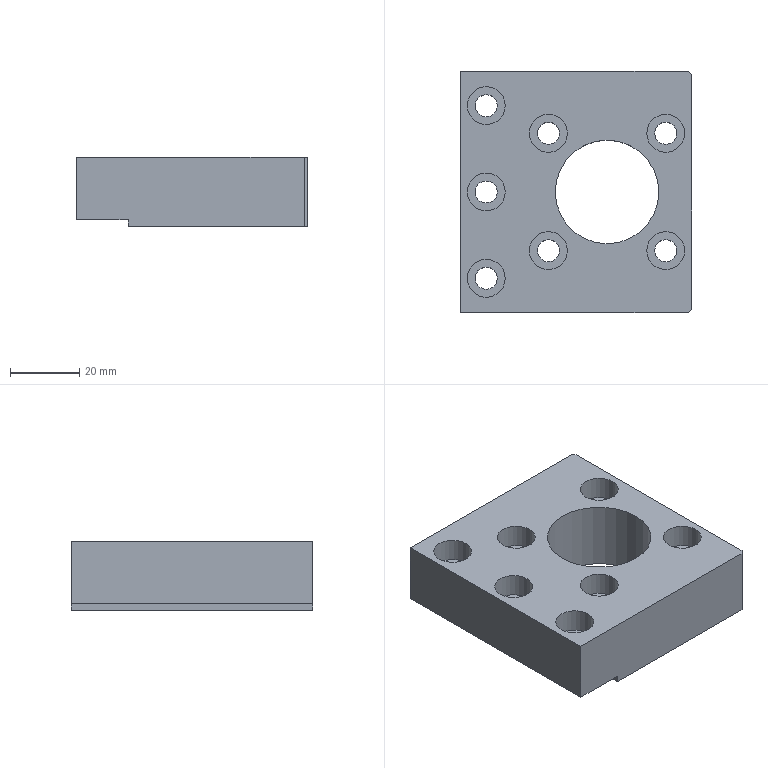Part | NX | 1 solid | 32 faces | box 67 x 70 x 20 mm | volume 70240 mm3 | plane 17 | cylinder 15 | commonest cylinder face diameters 6.4 x7 11 x7 30 x1
STEP:
#1=CARTESIAN_POINT('',(33.5,-34.,-10.));
#2=VERTEX_POINT('',#1);
#3=CARTESIAN_POINT('',(33.5,34.,-10.));
#4=VERTEX_POINT('',#3);
#5=CARTESIAN_POINT('',(33.5,35.,-10.));
#6=DIRECTION('',(0.,1.,0.));
#7=VECTOR('',#6,1000.);
#8=LINE('',#5,#7);
#9=EDGE_CURVE('',#2,#4,#8,.T.);
#10=ORIENTED_EDGE('',*,*,#9,.T.);
#11=CARTESIAN_POINT('',(33.5,34.,10.));
#12=VERTEX_POINT('',#11);
#13=CARTESIAN_POINT('',(33.5,34.,10.));
#14=DIRECTION('',(0.,0.,1.));
#15=VECTOR('',#14,1000.);
#16=LINE('',#13,#15);
#17=EDGE_CURVE('',#4,#12,#16,.T.);
#18=ORIENTED_EDGE('',*,*,#17,.T.);
#19=CARTESIAN_POINT('',(33.5,-34.,10.));
#20=VERTEX_POINT('',#19);
#21=CARTESIAN_POINT('',(33.5,35.,10.));
#22=DIRECTION('',(0.,1.,0.));
#23=VECTOR('',#22,1000.);
#24=LINE('',#21,#23);
#25=EDGE_CURVE('',#20,#12,#24,.T.);
#26=ORIENTED_EDGE('',*,*,#25,.F.);
#27=CARTESIAN_POINT('',(33.5,-34.,10.));
#28=DIRECTION('',(0.,0.,-1.));
#29=VECTOR('',#28,1000.);
#30=LINE('',#27,#29);
#31=EDGE_CURVE('',#20,#2,#30,.T.);
#32=ORIENTED_EDGE('',*,*,#31,.T.);
#33=EDGE_LOOP('',(#10,#18,#26,#32));
#34=FACE_BOUND('',#33,.T.);
#35=CARTESIAN_POINT('',(33.5,35.,10.));
#36=DIRECTION('',(-1.,0.,0.));
#37=DIRECTION('',(0.,-1.,0.));
#38=AXIS2_PLACEMENT_3D('',#35,#36,#37);
#39=PLANE('',#38);
#40=ADVANCED_FACE('',(#34),#39,.F.);
#41=CARTESIAN_POINT('',(32.5,35.,-10.));
#42=VERTEX_POINT('',#41);
#43=CARTESIAN_POINT('',(-18.5,35.,-10.));
#44=VERTEX_POINT('',#43);
#45=CARTESIAN_POINT('',(-33.5,35.,-10.));
#46=DIRECTION('',(-1.,0.,0.));
#47=VECTOR('',#46,1000.);
#48=LINE('',#45,#47);
#49=EDGE_CURVE('',#42,#44,#48,.T.);
#50=ORIENTED_EDGE('',*,*,#49,.T.);
#51=CARTESIAN_POINT('',(-18.5,35.,-8.));
#52=VERTEX_POINT('',#51);
#53=CARTESIAN_POINT('',(-18.5,35.,-10.));
#54=DIRECTION('',(0.,0.,-1.));
#55=VECTOR('',#54,1000.);
#56=LINE('',#53,#55);
#57=EDGE_CURVE('',#52,#44,#56,.T.);
#58=ORIENTED_EDGE('',*,*,#57,.F.);
#59=CARTESIAN_POINT('',(-33.5,35.,-8.));
#60=VERTEX_POINT('',#59);
#61=CARTESIAN_POINT('',(-33.5,35.,-8.));
#62=DIRECTION('',(1.,0.,0.));
#63=VECTOR('',#62,1000.);
#64=LINE('',#61,#63);
#65=EDGE_CURVE('',#60,#52,#64,.T.);
#66=ORIENTED_EDGE('',*,*,#65,.F.);
#67=CARTESIAN_POINT('',(-33.5,35.,10.));
#68=VERTEX_POINT('',#67);
#69=CARTESIAN_POINT('',(-33.5,35.,10.));
#70=DIRECTION('',(0.,0.,-1.));
#71=VECTOR('',#70,1000.);
#72=LINE('',#69,#71);
#73=EDGE_CURVE('',#68,#60,#72,.T.);
#74=ORIENTED_EDGE('',*,*,#73,.F.);
#75=CARTESIAN_POINT('',(32.5,35.,10.));
#76=VERTEX_POINT('',#75);
#77=CARTESIAN_POINT('',(-33.5,35.,10.));
#78=DIRECTION('',(-1.,0.,0.));
#79=VECTOR('',#78,1000.);
#80=LINE('',#77,#79);
#81=EDGE_CURVE('',#76,#68,#80,.T.);
#82=ORIENTED_EDGE('',*,*,#81,.F.);
#83=CARTESIAN_POINT('',(32.5,35.,10.));
#84=DIRECTION('',(0.,0.,-1.));
#85=VECTOR('',#84,1000.);
#86=LINE('',#83,#85);
#87=EDGE_CURVE('',#76,#42,#86,.T.);
#88=ORIENTED_EDGE('',*,*,#87,.T.);
#89=EDGE_LOOP('',(#50,#58,#66,#74,#82,#88));
#90=FACE_BOUND('',#89,.T.);
#91=CARTESIAN_POINT('',(-33.5,35.,10.));
#92=DIRECTION('',(0.,-1.,0.));
#93=DIRECTION('',(0.,0.,-1.));
#94=AXIS2_PLACEMENT_3D('',#91,#92,#93);
#95=PLANE('',#94);
#96=ADVANCED_FACE('',(#90),#95,.F.);
#97=ORIENTED_EDGE('',*,*,#73,.T.);
#98=CARTESIAN_POINT('',(-33.5,-35.,-8.));
#99=VERTEX_POINT('',#98);
#100=CARTESIAN_POINT('',(-33.5,-35.,-8.));
#101=DIRECTION('',(0.,1.,0.));
#102=VECTOR('',#101,1000.);
#103=LINE('',#100,#102);
#104=EDGE_CURVE('',#99,#60,#103,.T.);
#105=ORIENTED_EDGE('',*,*,#104,.F.);
#106=CARTESIAN_POINT('',(-33.5,-35.,10.));
#107=VERTEX_POINT('',#106);
#108=CARTESIAN_POINT('',(-33.5,-35.,10.));
#109=DIRECTION('',(0.,0.,-1.));
#110=VECTOR('',#109,1000.);
#111=LINE('',#108,#110);
#112=EDGE_CURVE('',#107,#99,#111,.T.);
#113=ORIENTED_EDGE('',*,*,#112,.F.);
#114=CARTESIAN_POINT('',(-33.5,35.,10.));
#115=DIRECTION('',(0.,-1.,0.));
#116=VECTOR('',#115,1000.);
#117=LINE('',#114,#116);
#118=EDGE_CURVE('',#68,#107,#117,.T.);
#119=ORIENTED_EDGE('',*,*,#118,.F.);
#120=EDGE_LOOP('',(#97,#105,#113,#119));
#121=FACE_BOUND('',#120,.T.);
#122=CARTESIAN_POINT('',(-33.5,35.,10.));
#123=DIRECTION('',(1.,0.,0.));
#124=DIRECTION('',(0.,1.,0.));
#125=AXIS2_PLACEMENT_3D('',#122,#123,#124);
#126=PLANE('',#125);
#127=ADVANCED_FACE('',(#121),#126,.F.);
#128=CARTESIAN_POINT('',(-18.5,-35.,-8.));
#129=VERTEX_POINT('',#128);
#130=CARTESIAN_POINT('',(-33.5,-35.,-8.));
#131=DIRECTION('',(1.,0.,0.));
#132=VECTOR('',#131,1000.);
#133=LINE('',#130,#132);
#134=EDGE_CURVE('',#99,#129,#133,.T.);
#135=ORIENTED_EDGE('',*,*,#134,.T.);
#136=CARTESIAN_POINT('',(-18.5,-35.,-10.));
#137=VERTEX_POINT('',#136);
#138=CARTESIAN_POINT('',(-18.5,-35.,-10.));
#139=DIRECTION('',(0.,0.,-1.));
#140=VECTOR('',#139,1000.);
#141=LINE('',#138,#140);
#142=EDGE_CURVE('',#129,#137,#141,.T.);
#143=ORIENTED_EDGE('',*,*,#142,.T.);
#144=CARTESIAN_POINT('',(32.5,-35.,-10.));
#145=VERTEX_POINT('',#144);
#146=CARTESIAN_POINT('',(-33.5,-35.,-10.));
#147=DIRECTION('',(1.,0.,0.));
#148=VECTOR('',#147,1000.);
#149=LINE('',#146,#148);
#150=EDGE_CURVE('',#137,#145,#149,.T.);
#151=ORIENTED_EDGE('',*,*,#150,.T.);
#152=CARTESIAN_POINT('',(32.5,-35.,10.));
#153=VERTEX_POINT('',#152);
#154=CARTESIAN_POINT('',(32.5,-35.,10.));
#155=DIRECTION('',(0.,0.,1.));
#156=VECTOR('',#155,1000.);
#157=LINE('',#154,#156);
#158=EDGE_CURVE('',#145,#153,#157,.T.);
#159=ORIENTED_EDGE('',*,*,#158,.T.);
#160=CARTESIAN_POINT('',(-33.5,-35.,10.));
#161=DIRECTION('',(1.,0.,0.));
#162=VECTOR('',#161,1000.);
#163=LINE('',#160,#162);
#164=EDGE_CURVE('',#107,#153,#163,.T.);
#165=ORIENTED_EDGE('',*,*,#164,.F.);
#166=ORIENTED_EDGE('',*,*,#112,.T.);
#167=EDGE_LOOP('',(#135,#143,#151,#159,#165,#166));
#168=FACE_BOUND('',#167,.T.);
#169=CARTESIAN_POINT('',(-33.5,-35.,10.));
#170=DIRECTION('',(0.,1.,0.));
#171=DIRECTION('',(0.,0.,1.));
#172=AXIS2_PLACEMENT_3D('',#169,#170,#171);
#173=PLANE('',#172);
#174=ADVANCED_FACE('',(#168),#173,.F.);
#175=CARTESIAN_POINT('',(-20.5,25.,10.));
#176=VERTEX_POINT('',#175);
#177=CARTESIAN_POINT('',(-26.,25.,10.));
#178=DIRECTION('',(0.,0.,1.));
#179=DIRECTION('',(1.,0.,0.));
#180=AXIS2_PLACEMENT_3D('',#177,#178,#179);
#181=CIRCLE('',#180,5.5);
#182=EDGE_CURVE('',#176,#176,#181,.T.);
#183=ORIENTED_EDGE('',*,*,#182,.F.);
#184=EDGE_LOOP('',(#183));
#185=FACE_BOUND('',#184,.T.);
#186=CARTESIAN_POINT('',(-20.5,0.,10.));
#187=VERTEX_POINT('',#186);
#188=CARTESIAN_POINT('',(-26.,0.,10.));
#189=DIRECTION('',(0.,0.,1.));
#190=DIRECTION('',(1.,0.,0.));
#191=AXIS2_PLACEMENT_3D('',#188,#189,#190);
#192=CIRCLE('',#191,5.5);
#193=EDGE_CURVE('',#187,#187,#192,.T.);
#194=ORIENTED_EDGE('',*,*,#193,.F.);
#195=EDGE_LOOP('',(#194));
#196=FACE_BOUND('',#195,.T.);
#197=CARTESIAN_POINT('',(-20.5,-25.,10.));
#198=VERTEX_POINT('',#197);
#199=CARTESIAN_POINT('',(-26.,-25.,10.));
#200=DIRECTION('',(0.,0.,1.));
#201=DIRECTION('',(1.,0.,0.));
#202=AXIS2_PLACEMENT_3D('',#199,#200,#201);
#203=CIRCLE('',#202,5.5);
#204=EDGE_CURVE('',#198,#198,#203,.T.);
#205=ORIENTED_EDGE('',*,*,#204,.F.);
#206=EDGE_LOOP('',(#205));
#207=FACE_BOUND('',#206,.T.);
#208=CARTESIAN_POINT('',(-2.5,-17.,10.));
#209=VERTEX_POINT('',#208);
#210=CARTESIAN_POINT('',(-8.,-17.,10.));
#211=DIRECTION('',(0.,0.,1.));
#212=DIRECTION('',(1.,0.,0.));
#213=AXIS2_PLACEMENT_3D('',#210,#211,#212);
#214=CIRCLE('',#213,5.5);
#215=EDGE_CURVE('',#209,#209,#214,.T.);
#216=ORIENTED_EDGE('',*,*,#215,.F.);
#217=EDGE_LOOP('',(#216));
#218=FACE_BOUND('',#217,.T.);
#219=CARTESIAN_POINT('',(-2.5,17.,10.));
#220=VERTEX_POINT('',#219);
#221=CARTESIAN_POINT('',(-8.,17.,10.));
#222=DIRECTION('',(0.,0.,1.));
#223=DIRECTION('',(1.,0.,0.));
#224=AXIS2_PLACEMENT_3D('',#221,#222,#223);
#225=CIRCLE('',#224,5.5);
#226=EDGE_CURVE('',#220,#220,#225,.T.);
#227=ORIENTED_EDGE('',*,*,#226,.F.);
#228=EDGE_LOOP('',(#227));
#229=FACE_BOUND('',#228,.T.);
#230=CARTESIAN_POINT('',(31.5,17.,10.));
#231=VERTEX_POINT('',#230);
#232=CARTESIAN_POINT('',(26.,17.,10.));
#233=DIRECTION('',(0.,0.,1.));
#234=DIRECTION('',(1.,0.,0.));
#235=AXIS2_PLACEMENT_3D('',#232,#233,#234);
#236=CIRCLE('',#235,5.5);
#237=EDGE_CURVE('',#231,#231,#236,.T.);
#238=ORIENTED_EDGE('',*,*,#237,.F.);
#239=EDGE_LOOP('',(#238));
#240=FACE_BOUND('',#239,.T.);
#241=CARTESIAN_POINT('',(31.5,-17.,10.));
#242=VERTEX_POINT('',#241);
#243=CARTESIAN_POINT('',(26.,-17.,10.));
#244=DIRECTION('',(0.,0.,1.));
#245=DIRECTION('',(1.,0.,0.));
#246=AXIS2_PLACEMENT_3D('',#243,#244,#245);
#247=CIRCLE('',#246,5.5);
#248=EDGE_CURVE('',#242,#242,#247,.T.);
#249=ORIENTED_EDGE('',*,*,#248,.F.);
#250=EDGE_LOOP('',(#249));
#251=FACE_BOUND('',#250,.T.);
#252=CARTESIAN_POINT('',(-6.,0.,10.));
#253=VERTEX_POINT('',#252);
#254=CARTESIAN_POINT('',(9.,0.,10.));
#255=DIRECTION('',(0.,0.,-1.));
#256=DIRECTION('',(-1.,0.,0.));
#257=AXIS2_PLACEMENT_3D('',#254,#255,#256);
#258=CIRCLE('',#257,15.);
#259=EDGE_CURVE('',#253,#253,#258,.T.);
#260=ORIENTED_EDGE('',*,*,#259,.T.);
#261=EDGE_LOOP('',(#260));
#262=FACE_BOUND('',#261,.T.);
#263=ORIENTED_EDGE('',*,*,#25,.T.);
#264=CARTESIAN_POINT('',(33.75,33.75,10.));
#265=DIRECTION('',(0.7071,-0.7071,0.));
#266=VECTOR('',#265,1000.);
#267=LINE('',#264,#266);
#268=EDGE_CURVE('',#12,#76,#267,.F.);
#269=ORIENTED_EDGE('',*,*,#268,.T.);
#270=ORIENTED_EDGE('',*,*,#81,.T.);
#271=ORIENTED_EDGE('',*,*,#118,.T.);
#272=ORIENTED_EDGE('',*,*,#164,.T.);
#273=CARTESIAN_POINT('',(33.75,-33.75,10.));
#274=DIRECTION('',(-0.7071,-0.7071,0.));
#275=VECTOR('',#274,1000.);
#276=LINE('',#273,#275);
#277=EDGE_CURVE('',#153,#20,#276,.F.);
#278=ORIENTED_EDGE('',*,*,#277,.T.);
#279=EDGE_LOOP('',(#263,#269,#270,#271,#272,#278));
#280=FACE_BOUND('',#279,.T.);
#281=CARTESIAN_POINT('',(0.,0.,10.));
#282=DIRECTION('',(0.,0.,1.));
#283=DIRECTION('',(1.,0.,0.));
#284=AXIS2_PLACEMENT_3D('',#281,#282,#283);
#285=PLANE('',#284);
#286=ADVANCED_FACE('',(#185,#196,#207,#218,#229,#240,#251,#262,#280),#285,.T.);
#287=CARTESIAN_POINT('',(-4.8,-17.,-10.));
#288=VERTEX_POINT('',#287);
#289=CARTESIAN_POINT('',(-8.,-17.,-10.));
#290=DIRECTION('',(0.,0.,1.));
#291=DIRECTION('',(1.,0.,0.));
#292=AXIS2_PLACEMENT_3D('',#289,#290,#291);
#293=CIRCLE('',#292,3.2);
#294=EDGE_CURVE('',#288,#288,#293,.T.);
#295=ORIENTED_EDGE('',*,*,#294,.T.);
#296=EDGE_LOOP('',(#295));
#297=FACE_BOUND('',#296,.T.);
#298=CARTESIAN_POINT('',(-4.8,17.,-10.));
#299=VERTEX_POINT('',#298);
#300=CARTESIAN_POINT('',(-8.,17.,-10.));
#301=DIRECTION('',(0.,0.,1.));
#302=DIRECTION('',(1.,0.,0.));
#303=AXIS2_PLACEMENT_3D('',#300,#301,#302);
#304=CIRCLE('',#303,3.2);
#305=EDGE_CURVE('',#299,#299,#304,.T.);
#306=ORIENTED_EDGE('',*,*,#305,.T.);
#307=EDGE_LOOP('',(#306));
#308=FACE_BOUND('',#307,.T.);
#309=CARTESIAN_POINT('',(29.2,17.,-10.));
#310=VERTEX_POINT('',#309);
#311=CARTESIAN_POINT('',(26.,17.,-10.));
#312=DIRECTION('',(0.,0.,1.));
#313=DIRECTION('',(1.,0.,0.));
#314=AXIS2_PLACEMENT_3D('',#311,#312,#313);
#315=CIRCLE('',#314,3.2);
#316=EDGE_CURVE('',#310,#310,#315,.T.);
#317=ORIENTED_EDGE('',*,*,#316,.T.);
#318=EDGE_LOOP('',(#317));
#319=FACE_BOUND('',#318,.T.);
#320=CARTESIAN_POINT('',(29.2,-17.,-10.));
#321=VERTEX_POINT('',#320);
#322=CARTESIAN_POINT('',(26.,-17.,-10.));
#323=DIRECTION('',(0.,0.,1.));
#324=DIRECTION('',(1.,0.,0.));
#325=AXIS2_PLACEMENT_3D('',#322,#323,#324);
#326=CIRCLE('',#325,3.2);
#327=EDGE_CURVE('',#321,#321,#326,.T.);
#328=ORIENTED_EDGE('',*,*,#327,.T.);
#329=EDGE_LOOP('',(#328));
#330=FACE_BOUND('',#329,.T.);
#331=CARTESIAN_POINT('',(-6.,0.,-10.));
#332=VERTEX_POINT('',#331);
#333=CARTESIAN_POINT('',(9.,0.,-10.));
#334=DIRECTION('',(0.,0.,-1.));
#335=DIRECTION('',(-1.,0.,0.));
#336=AXIS2_PLACEMENT_3D('',#333,#334,#335);
#337=CIRCLE('',#336,15.);
#338=EDGE_CURVE('',#332,#332,#337,.T.);
#339=ORIENTED_EDGE('',*,*,#338,.F.);
#340=EDGE_LOOP('',(#339));
#341=FACE_BOUND('',#340,.T.);
#342=ORIENTED_EDGE('',*,*,#150,.F.);
#343=CARTESIAN_POINT('',(-18.5,-35.,-10.));
#344=DIRECTION('',(0.,1.,0.));
#345=VECTOR('',#344,1000.);
#346=LINE('',#343,#345);
#347=EDGE_CURVE('',#137,#44,#346,.T.);
#348=ORIENTED_EDGE('',*,*,#347,.T.);
#349=ORIENTED_EDGE('',*,*,#49,.F.);
#350=CARTESIAN_POINT('',(32.5,35.,-10.));
#351=DIRECTION('',(-0.7071,0.7071,0.));
#352=VECTOR('',#351,1000.);
#353=LINE('',#350,#352);
#354=EDGE_CURVE('',#42,#4,#353,.F.);
#355=ORIENTED_EDGE('',*,*,#354,.T.);
#356=ORIENTED_EDGE('',*,*,#9,.F.);
#357=CARTESIAN_POINT('',(33.5,-34.,-10.));
#358=DIRECTION('',(0.7071,0.7071,0.));
#359=VECTOR('',#358,1000.);
#360=LINE('',#357,#359);
#361=EDGE_CURVE('',#2,#145,#360,.F.);
#362=ORIENTED_EDGE('',*,*,#361,.T.);
#363=EDGE_LOOP('',(#342,#348,#349,#355,#356,#362));
#364=FACE_BOUND('',#363,.T.);
#365=CARTESIAN_POINT('',(0.,0.,-10.));
#366=DIRECTION('',(0.,0.,1.));
#367=DIRECTION('',(1.,0.,0.));
#368=AXIS2_PLACEMENT_3D('',#365,#366,#367);
#369=PLANE('',#368);
#370=ADVANCED_FACE('',(#297,#308,#319,#330,#341,#364),#369,.F.);
#371=ORIENTED_EDGE('',*,*,#259,.F.);
#372=EDGE_LOOP('',(#371));
#373=FACE_BOUND('',#372,.T.);
#374=ORIENTED_EDGE('',*,*,#338,.T.);
#375=EDGE_LOOP('',(#374));
#376=FACE_BOUND('',#375,.T.);
#377=CARTESIAN_POINT('',(9.,0.,10.));
#378=DIRECTION('',(0.,0.,-1.));
#379=DIRECTION('',(-1.,0.,0.));
#380=AXIS2_PLACEMENT_3D('',#377,#378,#379);
#381=CYLINDRICAL_SURFACE('',#380,15.);
#382=ADVANCED_FACE('',(#373,#376),#381,.F.);
#383=ORIENTED_EDGE('',*,*,#268,.F.);
#384=ORIENTED_EDGE('',*,*,#17,.F.);
#385=ORIENTED_EDGE('',*,*,#354,.F.);
#386=ORIENTED_EDGE('',*,*,#87,.F.);
#387=EDGE_LOOP('',(#383,#384,#385,#386));
#388=FACE_BOUND('',#387,.T.);
#389=CARTESIAN_POINT('',(32.5,35.,10.));
#390=DIRECTION('',(-0.7071,-0.7071,0.));
#391=DIRECTION('',(0.,0.,-1.));
#392=AXIS2_PLACEMENT_3D('',#389,#390,#391);
#393=PLANE('',#392);
#394=ADVANCED_FACE('',(#388),#393,.F.);
#395=ORIENTED_EDGE('',*,*,#277,.F.);
#396=ORIENTED_EDGE('',*,*,#158,.F.);
#397=ORIENTED_EDGE('',*,*,#361,.F.);
#398=ORIENTED_EDGE('',*,*,#31,.F.);
#399=EDGE_LOOP('',(#395,#396,#397,#398));
#400=FACE_BOUND('',#399,.T.);
#401=CARTESIAN_POINT('',(33.5,-34.,10.));
#402=DIRECTION('',(-0.7071,0.7071,0.));
#403=DIRECTION('',(0.,0.,-1.));
#404=AXIS2_PLACEMENT_3D('',#401,#402,#403);
#405=PLANE('',#404);
#406=ADVANCED_FACE('',(#400),#405,.F.);
#407=ORIENTED_EDGE('',*,*,#327,.F.);
#408=EDGE_LOOP('',(#407));
#409=FACE_BOUND('',#408,.T.);
#410=CARTESIAN_POINT('',(29.2,-17.,3.2));
#411=VERTEX_POINT('',#410);
#412=CARTESIAN_POINT('',(26.,-17.,3.2));
#413=DIRECTION('',(0.,0.,1.));
#414=DIRECTION('',(1.,0.,0.));
#415=AXIS2_PLACEMENT_3D('',#412,#413,#414);
#416=CIRCLE('',#415,3.2);
#417=EDGE_CURVE('',#411,#411,#416,.T.);
#418=ORIENTED_EDGE('',*,*,#417,.T.);
#419=EDGE_LOOP('',(#418));
#420=FACE_BOUND('',#419,.T.);
#421=CARTESIAN_POINT('',(26.,-17.,10.));
#422=DIRECTION('',(0.,0.,1.));
#423=DIRECTION('',(1.,0.,0.));
#424=AXIS2_PLACEMENT_3D('',#421,#422,#423);
#425=CYLINDRICAL_SURFACE('',#424,3.2);
#426=ADVANCED_FACE('',(#409,#420),#425,.F.);
#427=ORIENTED_EDGE('',*,*,#417,.F.);
#428=EDGE_LOOP('',(#427));
#429=FACE_BOUND('',#428,.T.);
#430=CARTESIAN_POINT('',(31.5,-17.,3.2));
#431=VERTEX_POINT('',#430);
#432=CARTESIAN_POINT('',(26.,-17.,3.2));
#433=DIRECTION('',(0.,0.,1.));
#434=DIRECTION('',(1.,0.,0.));
#435=AXIS2_PLACEMENT_3D('',#432,#433,#434);
#436=CIRCLE('',#435,5.5);
#437=EDGE_CURVE('',#431,#431,#436,.T.);
#438=ORIENTED_EDGE('',*,*,#437,.T.);
#439=EDGE_LOOP('',(#438));
#440=FACE_BOUND('',#439,.T.);
#441=CARTESIAN_POINT('',(29.2,-17.,3.2));
#442=DIRECTION('',(0.,0.,-1.));
#443=DIRECTION('',(-1.,0.,0.));
#444=AXIS2_PLACEMENT_3D('',#441,#442,#443);
#445=PLANE('',#444);
#446=ADVANCED_FACE('',(#429,#440),#445,.F.);
#447=ORIENTED_EDGE('',*,*,#437,.F.);
#448=EDGE_LOOP('',(#447));
#449=FACE_BOUND('',#448,.T.);
#450=ORIENTED_EDGE('',*,*,#248,.T.);
#451=EDGE_LOOP('',(#450));
#452=FACE_BOUND('',#451,.T.);
#453=CARTESIAN_POINT('',(26.,-17.,10.));
#454=DIRECTION('',(0.,0.,1.));
#455=DIRECTION('',(1.,0.,0.));
#456=AXIS2_PLACEMENT_3D('',#453,#454,#455);
#457=CYLINDRICAL_SURFACE('',#456,5.5);
#458=ADVANCED_FACE('',(#449,#452),#457,.F.);
#459=ORIENTED_EDGE('',*,*,#316,.F.);
#460=EDGE_LOOP('',(#459));
#461=FACE_BOUND('',#460,.T.);
#462=CARTESIAN_POINT('',(29.2,17.,3.2));
#463=VERTEX_POINT('',#462);
#464=CARTESIAN_POINT('',(26.,17.,3.2));
#465=DIRECTION('',(0.,0.,1.));
#466=DIRECTION('',(1.,0.,0.));
#467=AXIS2_PLACEMENT_3D('',#464,#465,#466);
#468=CIRCLE('',#467,3.2);
#469=EDGE_CURVE('',#463,#463,#468,.T.);
#470=ORIENTED_EDGE('',*,*,#469,.T.);
#471=EDGE_LOOP('',(#470));
#472=FACE_BOUND('',#471,.T.);
#473=CARTESIAN_POINT('',(26.,17.,10.));
#474=DIRECTION('',(0.,0.,1.));
#475=DIRECTION('',(1.,0.,0.));
#476=AXIS2_PLACEMENT_3D('',#473,#474,#475);
#477=CYLINDRICAL_SURFACE('',#476,3.2);
#478=ADVANCED_FACE('',(#461,#472),#477,.F.);
#479=ORIENTED_EDGE('',*,*,#469,.F.);
#480=EDGE_LOOP('',(#479));
#481=FACE_BOUND('',#480,.T.);
#482=CARTESIAN_POINT('',(31.5,17.,3.2));
#483=VERTEX_POINT('',#482);
#484=CARTESIAN_POINT('',(26.,17.,3.2));
#485=DIRECTION('',(0.,0.,1.));
#486=DIRECTION('',(1.,0.,0.));
#487=AXIS2_PLACEMENT_3D('',#484,#485,#486);
#488=CIRCLE('',#487,5.5);
#489=EDGE_CURVE('',#483,#483,#488,.T.);
#490=ORIENTED_EDGE('',*,*,#489,.T.);
#491=EDGE_LOOP('',(#490));
#492=FACE_BOUND('',#491,.T.);
#493=CARTESIAN_POINT('',(29.2,17.,3.2));
#494=DIRECTION('',(0.,0.,-1.));
#495=DIRECTION('',(-1.,0.,0.));
#496=AXIS2_PLACEMENT_3D('',#493,#494,#495);
#497=PLANE('',#496);
#498=ADVANCED_FACE('',(#481,#492),#497,.F.);
#499=ORIENTED_EDGE('',*,*,#489,.F.);
#500=EDGE_LOOP('',(#499));
#501=FACE_BOUND('',#500,.T.);
#502=ORIENTED_EDGE('',*,*,#237,.T.);
#503=EDGE_LOOP('',(#502));
#504=FACE_BOUND('',#503,.T.);
#505=CARTESIAN_POINT('',(26.,17.,10.));
#506=DIRECTION('',(0.,0.,1.));
#507=DIRECTION('',(1.,0.,0.));
#508=AXIS2_PLACEMENT_3D('',#505,#506,#507);
#509=CYLINDRICAL_SURFACE('',#508,5.5);
#510=ADVANCED_FACE('',(#501,#504),#509,.F.);
#511=ORIENTED_EDGE('',*,*,#305,.F.);
#512=EDGE_LOOP('',(#511));
#513=FACE_BOUND('',#512,.T.);
#514=CARTESIAN_POINT('',(-4.8,17.,3.2));
#515=VERTEX_POINT('',#514);
#516=CARTESIAN_POINT('',(-8.,17.,3.2));
#517=DIRECTION('',(0.,0.,1.));
#518=DIRECTION('',(1.,0.,0.));
#519=AXIS2_PLACEMENT_3D('',#516,#517,#518);
#520=CIRCLE('',#519,3.2);
#521=EDGE_CURVE('',#515,#515,#520,.T.);
#522=ORIENTED_EDGE('',*,*,#521,.T.);
#523=EDGE_LOOP('',(#522));
#524=FACE_BOUND('',#523,.T.);
#525=CARTESIAN_POINT('',(-8.,17.,10.));
#526=DIRECTION('',(0.,0.,1.));
#527=DIRECTION('',(1.,0.,0.));
#528=AXIS2_PLACEMENT_3D('',#525,#526,#527);
#529=CYLINDRICAL_SURFACE('',#528,3.2);
#530=ADVANCED_FACE('',(#513,#524),#529,.F.);
#531=ORIENTED_EDGE('',*,*,#521,.F.);
#532=EDGE_LOOP('',(#531));
#533=FACE_BOUND('',#532,.T.);
#534=CARTESIAN_POINT('',(-2.5,17.,3.2));
#535=VERTEX_POINT('',#534);
#536=CARTESIAN_POINT('',(-8.,17.,3.2));
#537=DIRECTION('',(0.,0.,1.));
#538=DIRECTION('',(1.,0.,0.));
#539=AXIS2_PLACEMENT_3D('',#536,#537,#538);
#540=CIRCLE('',#539,5.5);
#541=EDGE_CURVE('',#535,#535,#540,.T.);
#542=ORIENTED_EDGE('',*,*,#541,.T.);
#543=EDGE_LOOP('',(#542));
#544=FACE_BOUND('',#543,.T.);
#545=CARTESIAN_POINT('',(-4.8,17.,3.2));
#546=DIRECTION('',(0.,0.,-1.));
#547=DIRECTION('',(-1.,0.,0.));
#548=AXIS2_PLACEMENT_3D('',#545,#546,#547);
#549=PLANE('',#548);
#550=ADVANCED_FACE('',(#533,#544),#549,.F.);
#551=ORIENTED_EDGE('',*,*,#541,.F.);
#552=EDGE_LOOP('',(#551));
#553=FACE_BOUND('',#552,.T.);
#554=ORIENTED_EDGE('',*,*,#226,.T.);
#555=EDGE_LOOP('',(#554));
#556=FACE_BOUND('',#555,.T.);
#557=CARTESIAN_POINT('',(-8.,17.,10.));
#558=DIRECTION('',(0.,0.,1.));
#559=DIRECTION('',(1.,0.,0.));
#560=AXIS2_PLACEMENT_3D('',#557,#558,#559);
#561=CYLINDRICAL_SURFACE('',#560,5.5);
#562=ADVANCED_FACE('',(#553,#556),#561,.F.);
#563=ORIENTED_EDGE('',*,*,#294,.F.);
#564=EDGE_LOOP('',(#563));
#565=FACE_BOUND('',#564,.T.);
#566=CARTESIAN_POINT('',(-4.8,-17.,3.2));
#567=VERTEX_POINT('',#566);
#568=CARTESIAN_POINT('',(-8.,-17.,3.2));
#569=DIRECTION('',(0.,0.,1.));
#570=DIRECTION('',(1.,0.,0.));
#571=AXIS2_PLACEMENT_3D('',#568,#569,#570);
#572=CIRCLE('',#571,3.2);
#573=EDGE_CURVE('',#567,#567,#572,.T.);
#574=ORIENTED_EDGE('',*,*,#573,.T.);
#575=EDGE_LOOP('',(#574));
#576=FACE_BOUND('',#575,.T.);
#577=CARTESIAN_POINT('',(-8.,-17.,10.));
#578=DIRECTION('',(0.,0.,1.));
#579=DIRECTION('',(1.,0.,0.));
#580=AXIS2_PLACEMENT_3D('',#577,#578,#579);
#581=CYLINDRICAL_SURFACE('',#580,3.2);
#582=ADVANCED_FACE('',(#565,#576),#581,.F.);
#583=ORIENTED_EDGE('',*,*,#573,.F.);
#584=EDGE_LOOP('',(#583));
#585=FACE_BOUND('',#584,.T.);
#586=CARTESIAN_POINT('',(-2.5,-17.,3.2));
#587=VERTEX_POINT('',#586);
#588=CARTESIAN_POINT('',(-8.,-17.,3.2));
#589=DIRECTION('',(0.,0.,1.));
#590=DIRECTION('',(1.,0.,0.));
#591=AXIS2_PLACEMENT_3D('',#588,#589,#590);
#592=CIRCLE('',#591,5.5);
#593=EDGE_CURVE('',#587,#587,#592,.T.);
#594=ORIENTED_EDGE('',*,*,#593,.T.);
#595=EDGE_LOOP('',(#594));
#596=FACE_BOUND('',#595,.T.);
#597=CARTESIAN_POINT('',(-4.8,-17.,3.2));
#598=DIRECTION('',(0.,0.,-1.));
#599=DIRECTION('',(-1.,0.,0.));
#600=AXIS2_PLACEMENT_3D('',#597,#598,#599);
#601=PLANE('',#600);
#602=ADVANCED_FACE('',(#585,#596),#601,.F.);
#603=ORIENTED_EDGE('',*,*,#593,.F.);
#604=EDGE_LOOP('',(#603));
#605=FACE_BOUND('',#604,.T.);
#606=ORIENTED_EDGE('',*,*,#215,.T.);
#607=EDGE_LOOP('',(#606));
#608=FACE_BOUND('',#607,.T.);
#609=CARTESIAN_POINT('',(-8.,-17.,10.));
#610=DIRECTION('',(0.,0.,1.));
#611=DIRECTION('',(1.,0.,0.));
#612=AXIS2_PLACEMENT_3D('',#609,#610,#611);
#613=CYLINDRICAL_SURFACE('',#612,5.5);
#614=ADVANCED_FACE('',(#605,#608),#613,.F.);
#615=ORIENTED_EDGE('',*,*,#57,.T.);
#616=ORIENTED_EDGE('',*,*,#347,.F.);
#617=ORIENTED_EDGE('',*,*,#142,.F.);
#618=CARTESIAN_POINT('',(-18.5,-35.,-8.));
#619=DIRECTION('',(0.,1.,0.));
#620=VECTOR('',#619,1000.);
#621=LINE('',#618,#620);
#622=EDGE_CURVE('',#129,#52,#621,.T.);
#623=ORIENTED_EDGE('',*,*,#622,.T.);
#624=EDGE_LOOP('',(#615,#616,#617,#623));
#625=FACE_BOUND('',#624,.T.);
#626=CARTESIAN_POINT('',(-18.5,-35.,-10.));
#627=DIRECTION('',(1.,0.,0.));
#628=DIRECTION('',(0.,0.,-1.));
#629=AXIS2_PLACEMENT_3D('',#626,#627,#628);
#630=PLANE('',#629);
#631=ADVANCED_FACE('',(#625),#630,.F.);
#632=CARTESIAN_POINT('',(-22.8,25.,-8.));
#633=VERTEX_POINT('',#632);
#634=CARTESIAN_POINT('',(-26.,25.,-8.));
#635=DIRECTION('',(0.,0.,1.));
#636=DIRECTION('',(1.,0.,0.));
#637=AXIS2_PLACEMENT_3D('',#634,#635,#636);
#638=CIRCLE('',#637,3.2);
#639=EDGE_CURVE('',#633,#633,#638,.T.);
#640=ORIENTED_EDGE('',*,*,#639,.T.);
#641=EDGE_LOOP('',(#640));
#642=FACE_BOUND('',#641,.T.);
#643=CARTESIAN_POINT('',(-22.8,0.,-8.));
#644=VERTEX_POINT('',#643);
#645=CARTESIAN_POINT('',(-26.,0.,-8.));
#646=DIRECTION('',(0.,0.,1.));
#647=DIRECTION('',(1.,0.,0.));
#648=AXIS2_PLACEMENT_3D('',#645,#646,#647);
#649=CIRCLE('',#648,3.2);
#650=EDGE_CURVE('',#644,#644,#649,.T.);
#651=ORIENTED_EDGE('',*,*,#650,.T.);
#652=EDGE_LOOP('',(#651));
#653=FACE_BOUND('',#652,.T.);
#654=CARTESIAN_POINT('',(-22.8,-25.,-8.));
#655=VERTEX_POINT('',#654);
#656=CARTESIAN_POINT('',(-26.,-25.,-8.));
#657=DIRECTION('',(0.,0.,1.));
#658=DIRECTION('',(1.,0.,0.));
#659=AXIS2_PLACEMENT_3D('',#656,#657,#658);
#660=CIRCLE('',#659,3.2);
#661=EDGE_CURVE('',#655,#655,#660,.T.);
#662=ORIENTED_EDGE('',*,*,#661,.T.);
#663=EDGE_LOOP('',(#662));
#664=FACE_BOUND('',#663,.T.);
#665=ORIENTED_EDGE('',*,*,#65,.T.);
#666=ORIENTED_EDGE('',*,*,#622,.F.);
#667=ORIENTED_EDGE('',*,*,#134,.F.);
#668=ORIENTED_EDGE('',*,*,#104,.T.);
#669=EDGE_LOOP('',(#665,#666,#667,#668));
#670=FACE_BOUND('',#669,.T.);
#671=CARTESIAN_POINT('',(-33.5,-35.,-8.));
#672=DIRECTION('',(0.,0.,1.));
#673=DIRECTION('',(1.,0.,0.));
#674=AXIS2_PLACEMENT_3D('',#671,#672,#673);
#675=PLANE('',#674);
#676=ADVANCED_FACE('',(#642,#653,#664,#670),#675,.F.);
#677=CARTESIAN_POINT('',(-22.8,-25.,3.2));
#678=VERTEX_POINT('',#677);
#679=CARTESIAN_POINT('',(-26.,-25.,3.2));
#680=DIRECTION('',(0.,0.,1.));
#681=DIRECTION('',(1.,0.,0.));
#682=AXIS2_PLACEMENT_3D('',#679,#680,#681);
#683=CIRCLE('',#682,3.2);
#684=EDGE_CURVE('',#678,#678,#683,.T.);
#685=ORIENTED_EDGE('',*,*,#684,.T.);
#686=EDGE_LOOP('',(#685));
#687=FACE_BOUND('',#686,.T.);
#688=ORIENTED_EDGE('',*,*,#661,.F.);
#689=EDGE_LOOP('',(#688));
#690=FACE_BOUND('',#689,.T.);
#691=CARTESIAN_POINT('',(-26.,-25.,10.));
#692=DIRECTION('',(0.,0.,1.));
#693=DIRECTION('',(1.,0.,0.));
#694=AXIS2_PLACEMENT_3D('',#691,#692,#693);
#695=CYLINDRICAL_SURFACE('',#694,3.2);
#696=ADVANCED_FACE('',(#687,#690),#695,.F.);
#697=ORIENTED_EDGE('',*,*,#684,.F.);
#698=EDGE_LOOP('',(#697));
#699=FACE_BOUND('',#698,.T.);
#700=CARTESIAN_POINT('',(-20.5,-25.,3.2));
#701=VERTEX_POINT('',#700);
#702=CARTESIAN_POINT('',(-26.,-25.,3.2));
#703=DIRECTION('',(0.,0.,1.));
#704=DIRECTION('',(1.,0.,0.));
#705=AXIS2_PLACEMENT_3D('',#702,#703,#704);
#706=CIRCLE('',#705,5.5);
#707=EDGE_CURVE('',#701,#701,#706,.T.);
#708=ORIENTED_EDGE('',*,*,#707,.T.);
#709=EDGE_LOOP('',(#708));
#710=FACE_BOUND('',#709,.T.);
#711=CARTESIAN_POINT('',(-22.8,-25.,3.2));
#712=DIRECTION('',(0.,0.,-1.));
#713=DIRECTION('',(-1.,0.,0.));
#714=AXIS2_PLACEMENT_3D('',#711,#712,#713);
#715=PLANE('',#714);
#716=ADVANCED_FACE('',(#699,#710),#715,.F.);
#717=ORIENTED_EDGE('',*,*,#707,.F.);
#718=EDGE_LOOP('',(#717));
#719=FACE_BOUND('',#718,.T.);
#720=ORIENTED_EDGE('',*,*,#204,.T.);
#721=EDGE_LOOP('',(#720));
#722=FACE_BOUND('',#721,.T.);
#723=CARTESIAN_POINT('',(-26.,-25.,10.));
#724=DIRECTION('',(0.,0.,1.));
#725=DIRECTION('',(1.,0.,0.));
#726=AXIS2_PLACEMENT_3D('',#723,#724,#725);
#727=CYLINDRICAL_SURFACE('',#726,5.5);
#728=ADVANCED_FACE('',(#719,#722),#727,.F.);
#729=CARTESIAN_POINT('',(-22.8,0.,3.2));
#730=VERTEX_POINT('',#729);
#731=CARTESIAN_POINT('',(-26.,0.,3.2));
#732=DIRECTION('',(0.,0.,1.));
#733=DIRECTION('',(1.,0.,0.));
#734=AXIS2_PLACEMENT_3D('',#731,#732,#733);
#735=CIRCLE('',#734,3.2);
#736=EDGE_CURVE('',#730,#730,#735,.T.);
#737=ORIENTED_EDGE('',*,*,#736,.T.);
#738=EDGE_LOOP('',(#737));
#739=FACE_BOUND('',#738,.T.);
#740=ORIENTED_EDGE('',*,*,#650,.F.);
#741=EDGE_LOOP('',(#740));
#742=FACE_BOUND('',#741,.T.);
#743=CARTESIAN_POINT('',(-26.,0.,10.));
#744=DIRECTION('',(0.,0.,1.));
#745=DIRECTION('',(1.,0.,0.));
#746=AXIS2_PLACEMENT_3D('',#743,#744,#745);
#747=CYLINDRICAL_SURFACE('',#746,3.2);
#748=ADVANCED_FACE('',(#739,#742),#747,.F.);
#749=ORIENTED_EDGE('',*,*,#736,.F.);
#750=EDGE_LOOP('',(#749));
#751=FACE_BOUND('',#750,.T.);
#752=CARTESIAN_POINT('',(-20.5,0.,3.2));
#753=VERTEX_POINT('',#752);
#754=CARTESIAN_POINT('',(-26.,0.,3.2));
#755=DIRECTION('',(0.,0.,1.));
#756=DIRECTION('',(1.,0.,0.));
#757=AXIS2_PLACEMENT_3D('',#754,#755,#756);
#758=CIRCLE('',#757,5.5);
#759=EDGE_CURVE('',#753,#753,#758,.T.);
#760=ORIENTED_EDGE('',*,*,#759,.T.);
#761=EDGE_LOOP('',(#760));
#762=FACE_BOUND('',#761,.T.);
#763=CARTESIAN_POINT('',(-22.8,0.,3.2));
#764=DIRECTION('',(0.,0.,-1.));
#765=DIRECTION('',(-1.,0.,0.));
#766=AXIS2_PLACEMENT_3D('',#763,#764,#765);
#767=PLANE('',#766);
#768=ADVANCED_FACE('',(#751,#762),#767,.F.);
#769=ORIENTED_EDGE('',*,*,#759,.F.);
#770=EDGE_LOOP('',(#769));
#771=FACE_BOUND('',#770,.T.);
#772=ORIENTED_EDGE('',*,*,#193,.T.);
#773=EDGE_LOOP('',(#772));
#774=FACE_BOUND('',#773,.T.);
#775=CARTESIAN_POINT('',(-26.,0.,10.));
#776=DIRECTION('',(0.,0.,1.));
#777=DIRECTION('',(1.,0.,0.));
#778=AXIS2_PLACEMENT_3D('',#775,#776,#777);
#779=CYLINDRICAL_SURFACE('',#778,5.5);
#780=ADVANCED_FACE('',(#771,#774),#779,.F.);
#781=CARTESIAN_POINT('',(-22.8,25.,3.2));
#782=VERTEX_POINT('',#781);
#783=CARTESIAN_POINT('',(-26.,25.,3.2));
#784=DIRECTION('',(0.,0.,1.));
#785=DIRECTION('',(1.,0.,0.));
#786=AXIS2_PLACEMENT_3D('',#783,#784,#785);
#787=CIRCLE('',#786,3.2);
#788=EDGE_CURVE('',#782,#782,#787,.T.);
#789=ORIENTED_EDGE('',*,*,#788,.T.);
#790=EDGE_LOOP('',(#789));
#791=FACE_BOUND('',#790,.T.);
#792=ORIENTED_EDGE('',*,*,#639,.F.);
#793=EDGE_LOOP('',(#792));
#794=FACE_BOUND('',#793,.T.);
#795=CARTESIAN_POINT('',(-26.,25.,10.));
#796=DIRECTION('',(0.,0.,1.));
#797=DIRECTION('',(1.,0.,0.));
#798=AXIS2_PLACEMENT_3D('',#795,#796,#797);
#799=CYLINDRICAL_SURFACE('',#798,3.2);
#800=ADVANCED_FACE('',(#791,#794),#799,.F.);
#801=ORIENTED_EDGE('',*,*,#788,.F.);
#802=EDGE_LOOP('',(#801));
#803=FACE_BOUND('',#802,.T.);
#804=CARTESIAN_POINT('',(-20.5,25.,3.2));
#805=VERTEX_POINT('',#804);
#806=CARTESIAN_POINT('',(-26.,25.,3.2));
#807=DIRECTION('',(0.,0.,1.));
#808=DIRECTION('',(1.,0.,0.));
#809=AXIS2_PLACEMENT_3D('',#806,#807,#808);
#810=CIRCLE('',#809,5.5);
#811=EDGE_CURVE('',#805,#805,#810,.T.);
#812=ORIENTED_EDGE('',*,*,#811,.T.);
#813=EDGE_LOOP('',(#812));
#814=FACE_BOUND('',#813,.T.);
#815=CARTESIAN_POINT('',(-22.8,25.,3.2));
#816=DIRECTION('',(0.,0.,-1.));
#817=DIRECTION('',(-1.,0.,0.));
#818=AXIS2_PLACEMENT_3D('',#815,#816,#817);
#819=PLANE('',#818);
#820=ADVANCED_FACE('',(#803,#814),#819,.F.);
#821=ORIENTED_EDGE('',*,*,#811,.F.);
#822=EDGE_LOOP('',(#821));
#823=FACE_BOUND('',#822,.T.);
#824=ORIENTED_EDGE('',*,*,#182,.T.);
#825=EDGE_LOOP('',(#824));
#826=FACE_BOUND('',#825,.T.);
#827=CARTESIAN_POINT('',(-26.,25.,10.));
#828=DIRECTION('',(0.,0.,1.));
#829=DIRECTION('',(1.,0.,0.));
#830=AXIS2_PLACEMENT_3D('',#827,#828,#829);
#831=CYLINDRICAL_SURFACE('',#830,5.5);
#832=ADVANCED_FACE('',(#823,#826),#831,.F.);
#833=CLOSED_SHELL('',(#40,#96,#127,#174,#286,#370,#382,#394,#406,#426,#446,#458,#478,#498,#510,#530,#550,#562,#582,#602,#614,#631,#676,#696,#716,#728,#748,#768,#780,#800,#820,#832));
#834=MANIFOLD_SOLID_BREP('',#833);
#835=(LENGTH_UNIT()NAMED_UNIT(*)SI_UNIT(.MILLI.,.METRE.));
#836=UNCERTAINTY_MEASURE_WITH_UNIT(LENGTH_MEASURE(0.00001),#835,'','');
#837=(NAMED_UNIT(*)PLANE_ANGLE_UNIT()SI_UNIT($,.RADIAN.));
#838=(NAMED_UNIT(*)SI_UNIT($,.STERADIAN.)SOLID_ANGLE_UNIT());
#839=(GEOMETRIC_REPRESENTATION_CONTEXT(3)GLOBAL_UNCERTAINTY_ASSIGNED_CONTEXT((#836))GLOBAL_UNIT_ASSIGNED_CONTEXT((#835,#837,#838))REPRESENTATION_CONTEXT('',''));
#840=ADVANCED_BREP_SHAPE_REPRESENTATION('',(#834),#839);